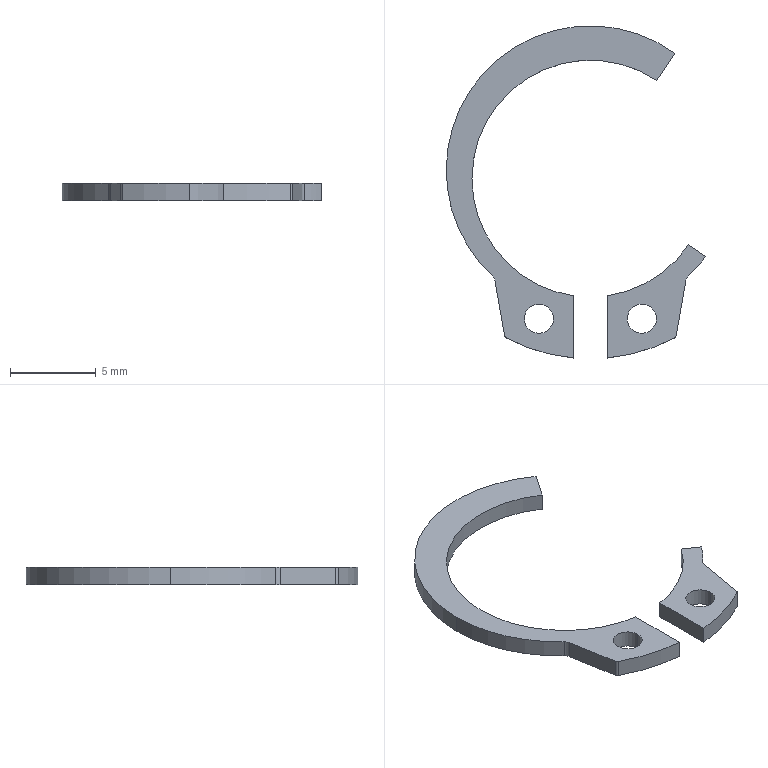Part | STEP file | Shaft retaining ring type A 15 | 2 solids | 26 faces | box 15.123 x 19.352 x 1 mm | volume 70.172 mm3 | cylinder 16 | plane 10 | commonest cylinder face diameters 1.7 x4 13.8 x3 16.8 x3 0.4 x2 1 x2 21 x2